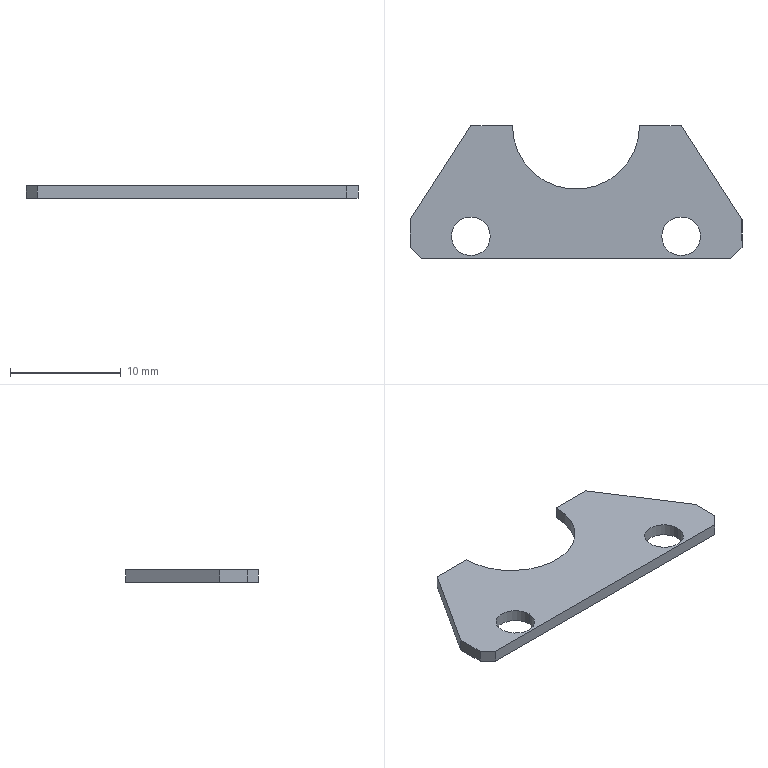Part | STEP file | 11-FG-SB00511 | 1 solid | 16 faces | box 30 x 12 x 1.1 mm | volume 265.181 mm3 | plane 11 | cylinder 5 | commonest cylinder face diameters 3.5 x4 11.5 x1
STEP:
#1=CARTESIAN_POINT('',(11.25,-4.,1.1));
#2=VERTEX_POINT('',#1);
#3=CARTESIAN_POINT('',(7.75,-4.,1.1));
#4=VERTEX_POINT('',#3);
#5=CARTESIAN_POINT('',(9.5,-4.,1.1));
#6=DIRECTION('',(0.,0.,-1.));
#7=DIRECTION('',(1.,0.,0.));
#8=AXIS2_PLACEMENT_3D('',#5,#6,#7);
#9=CIRCLE('',#8,1.75);
#10=EDGE_CURVE('',#2,#4,#9,.T.);
#11=ORIENTED_EDGE('',*,*,#10,.F.);
#12=CARTESIAN_POINT('',(11.25,-4.,0.));
#13=VERTEX_POINT('',#12);
#14=CARTESIAN_POINT('',(11.25,-4.,1.1));
#15=DIRECTION('',(0.,0.,-1.));
#16=VECTOR('',#15,1000.);
#17=LINE('',#14,#16);
#18=EDGE_CURVE('',#2,#13,#17,.T.);
#19=ORIENTED_EDGE('',*,*,#18,.T.);
#20=CARTESIAN_POINT('',(7.75,-4.,0.));
#21=VERTEX_POINT('',#20);
#22=CARTESIAN_POINT('',(9.5,-4.,0.));
#23=DIRECTION('',(0.,0.,1.));
#24=DIRECTION('',(1.,0.,0.));
#25=AXIS2_PLACEMENT_3D('',#22,#23,#24);
#26=CIRCLE('',#25,1.75);
#27=EDGE_CURVE('',#21,#13,#26,.T.);
#28=ORIENTED_EDGE('',*,*,#27,.F.);
#29=CARTESIAN_POINT('',(7.75,-4.,1.1));
#30=DIRECTION('',(0.,0.,-1.));
#31=VECTOR('',#30,1000.);
#32=LINE('',#29,#31);
#33=EDGE_CURVE('',#4,#21,#32,.T.);
#34=ORIENTED_EDGE('',*,*,#33,.F.);
#35=EDGE_LOOP('',(#11,#19,#28,#34));
#36=FACE_OUTER_BOUND('',#35,.T.);
#37=CARTESIAN_POINT('',(9.5,-4.,1.1));
#38=DIRECTION('',(0.,0.,-1.));
#39=DIRECTION('',(-1.,0.,0.));
#40=AXIS2_PLACEMENT_3D('',#37,#38,#39);
#41=CYLINDRICAL_SURFACE('',#40,1.75);
#42=ADVANCED_FACE('',(#36),#41,.F.);
#43=CARTESIAN_POINT('',(-7.75,-4.,1.1));
#44=VERTEX_POINT('',#43);
#45=CARTESIAN_POINT('',(-11.25,-4.,1.1));
#46=VERTEX_POINT('',#45);
#47=CARTESIAN_POINT('',(-9.5,-4.,1.1));
#48=DIRECTION('',(0.,0.,-1.));
#49=DIRECTION('',(-1.,0.,0.));
#50=AXIS2_PLACEMENT_3D('',#47,#48,#49);
#51=CIRCLE('',#50,1.75);
#52=EDGE_CURVE('',#44,#46,#51,.T.);
#53=ORIENTED_EDGE('',*,*,#52,.F.);
#54=CARTESIAN_POINT('',(-7.75,-4.,0.));
#55=VERTEX_POINT('',#54);
#56=CARTESIAN_POINT('',(-7.75,-4.,1.1));
#57=DIRECTION('',(0.,0.,-1.));
#58=VECTOR('',#57,1000.);
#59=LINE('',#56,#58);
#60=EDGE_CURVE('',#44,#55,#59,.T.);
#61=ORIENTED_EDGE('',*,*,#60,.T.);
#62=CARTESIAN_POINT('',(-11.25,-4.,0.));
#63=VERTEX_POINT('',#62);
#64=CARTESIAN_POINT('',(-9.5,-4.,0.));
#65=DIRECTION('',(0.,0.,1.));
#66=DIRECTION('',(1.,0.,0.));
#67=AXIS2_PLACEMENT_3D('',#64,#65,#66);
#68=CIRCLE('',#67,1.75);
#69=EDGE_CURVE('',#63,#55,#68,.T.);
#70=ORIENTED_EDGE('',*,*,#69,.F.);
#71=CARTESIAN_POINT('',(-11.25,-4.,1.1));
#72=DIRECTION('',(0.,0.,-1.));
#73=VECTOR('',#72,1000.);
#74=LINE('',#71,#73);
#75=EDGE_CURVE('',#46,#63,#74,.T.);
#76=ORIENTED_EDGE('',*,*,#75,.F.);
#77=EDGE_LOOP('',(#53,#61,#70,#76));
#78=FACE_OUTER_BOUND('',#77,.T.);
#79=CARTESIAN_POINT('',(-9.5,-4.,1.1));
#80=DIRECTION('',(0.,0.,-1.));
#81=DIRECTION('',(-1.,0.,0.));
#82=AXIS2_PLACEMENT_3D('',#79,#80,#81);
#83=CYLINDRICAL_SURFACE('',#82,1.75);
#84=ADVANCED_FACE('',(#78),#83,.F.);
#85=CARTESIAN_POINT('',(9.5,6.,1.1));
#86=VERTEX_POINT('',#85);
#87=CARTESIAN_POINT('',(5.75,6.,1.1));
#88=VERTEX_POINT('',#87);
#89=CARTESIAN_POINT('',(-15.,6.,1.1));
#90=DIRECTION('',(-1.,0.,0.));
#91=VECTOR('',#90,1000.);
#92=LINE('',#89,#91);
#93=EDGE_CURVE('',#86,#88,#92,.T.);
#94=ORIENTED_EDGE('',*,*,#93,.F.);
#95=CARTESIAN_POINT('',(9.5,6.,0.));
#96=VERTEX_POINT('',#95);
#97=CARTESIAN_POINT('',(9.5,6.,1.1));
#98=DIRECTION('',(0.,0.,-1.));
#99=VECTOR('',#98,1000.);
#100=LINE('',#97,#99);
#101=EDGE_CURVE('',#86,#96,#100,.T.);
#102=ORIENTED_EDGE('',*,*,#101,.T.);
#103=CARTESIAN_POINT('',(5.75,6.,0.));
#104=VERTEX_POINT('',#103);
#105=CARTESIAN_POINT('',(-15.,6.,0.));
#106=DIRECTION('',(-1.,0.,0.));
#107=VECTOR('',#106,1000.);
#108=LINE('',#105,#107);
#109=EDGE_CURVE('',#96,#104,#108,.T.);
#110=ORIENTED_EDGE('',*,*,#109,.T.);
#111=CARTESIAN_POINT('',(5.75,6.,0.));
#112=DIRECTION('',(0.,0.,1.));
#113=VECTOR('',#112,1000.);
#114=LINE('',#111,#113);
#115=EDGE_CURVE('',#104,#88,#114,.T.);
#116=ORIENTED_EDGE('',*,*,#115,.T.);
#117=EDGE_LOOP('',(#94,#102,#110,#116));
#118=FACE_OUTER_BOUND('',#117,.T.);
#119=CARTESIAN_POINT('',(-15.,6.,1.1));
#120=DIRECTION('',(0.,-1.,0.));
#121=DIRECTION('',(0.,0.,-1.));
#122=AXIS2_PLACEMENT_3D('',#119,#120,#121);
#123=PLANE('',#122);
#124=ADVANCED_FACE('',(#118),#123,.F.);
#125=CARTESIAN_POINT('',(15.,-5.,0.));
#126=VERTEX_POINT('',#125);
#127=CARTESIAN_POINT('',(15.,-2.5,0.));
#128=VERTEX_POINT('',#127);
#129=CARTESIAN_POINT('',(15.,6.,0.));
#130=DIRECTION('',(0.,1.,0.));
#131=VECTOR('',#130,1000.);
#132=LINE('',#129,#131);
#133=EDGE_CURVE('',#126,#128,#132,.T.);
#134=ORIENTED_EDGE('',*,*,#133,.T.);
#135=CARTESIAN_POINT('',(15.,-2.5,1.1));
#136=VERTEX_POINT('',#135);
#137=CARTESIAN_POINT('',(15.,-2.5,1.1));
#138=DIRECTION('',(0.,0.,-1.));
#139=VECTOR('',#138,1000.);
#140=LINE('',#137,#139);
#141=EDGE_CURVE('',#136,#128,#140,.T.);
#142=ORIENTED_EDGE('',*,*,#141,.F.);
#143=CARTESIAN_POINT('',(15.,-5.,1.1));
#144=VERTEX_POINT('',#143);
#145=CARTESIAN_POINT('',(15.,6.,1.1));
#146=DIRECTION('',(0.,1.,0.));
#147=VECTOR('',#146,1000.);
#148=LINE('',#145,#147);
#149=EDGE_CURVE('',#144,#136,#148,.T.);
#150=ORIENTED_EDGE('',*,*,#149,.F.);
#151=CARTESIAN_POINT('',(15.,-5.,1.1));
#152=DIRECTION('',(0.,0.,-1.));
#153=VECTOR('',#152,1000.);
#154=LINE('',#151,#153);
#155=EDGE_CURVE('',#144,#126,#154,.T.);
#156=ORIENTED_EDGE('',*,*,#155,.T.);
#157=EDGE_LOOP('',(#134,#142,#150,#156));
#158=FACE_OUTER_BOUND('',#157,.T.);
#159=CARTESIAN_POINT('',(15.,6.,1.1));
#160=DIRECTION('',(-1.,0.,0.));
#161=DIRECTION('',(0.,-1.,0.));
#162=AXIS2_PLACEMENT_3D('',#159,#160,#161);
#163=PLANE('',#162);
#164=ADVANCED_FACE('',(#158),#163,.F.);
#165=CARTESIAN_POINT('',(-5.75,6.,0.));
#166=VERTEX_POINT('',#165);
#167=CARTESIAN_POINT('',(-9.5,6.,0.));
#168=VERTEX_POINT('',#167);
#169=CARTESIAN_POINT('',(-15.,6.,0.));
#170=DIRECTION('',(-1.,0.,0.));
#171=VECTOR('',#170,1000.);
#172=LINE('',#169,#171);
#173=EDGE_CURVE('',#166,#168,#172,.T.);
#174=ORIENTED_EDGE('',*,*,#173,.T.);
#175=CARTESIAN_POINT('',(-9.5,6.,1.1));
#176=VERTEX_POINT('',#175);
#177=CARTESIAN_POINT('',(-9.5,6.,1.1));
#178=DIRECTION('',(0.,0.,-1.));
#179=VECTOR('',#178,1000.);
#180=LINE('',#177,#179);
#181=EDGE_CURVE('',#176,#168,#180,.T.);
#182=ORIENTED_EDGE('',*,*,#181,.F.);
#183=CARTESIAN_POINT('',(-5.75,6.,1.1));
#184=VERTEX_POINT('',#183);
#185=CARTESIAN_POINT('',(-15.,6.,1.1));
#186=DIRECTION('',(-1.,0.,0.));
#187=VECTOR('',#186,1000.);
#188=LINE('',#185,#187);
#189=EDGE_CURVE('',#184,#176,#188,.T.);
#190=ORIENTED_EDGE('',*,*,#189,.F.);
#191=CARTESIAN_POINT('',(-5.75,6.,0.));
#192=DIRECTION('',(0.,0.,-1.));
#193=VECTOR('',#192,1000.);
#194=LINE('',#191,#193);
#195=EDGE_CURVE('',#184,#166,#194,.T.);
#196=ORIENTED_EDGE('',*,*,#195,.T.);
#197=EDGE_LOOP('',(#174,#182,#190,#196));
#198=FACE_OUTER_BOUND('',#197,.T.);
#199=CARTESIAN_POINT('',(-15.,6.,1.1));
#200=DIRECTION('',(0.,-1.,0.));
#201=DIRECTION('',(0.,0.,-1.));
#202=AXIS2_PLACEMENT_3D('',#199,#200,#201);
#203=PLANE('',#202);
#204=ADVANCED_FACE('',(#198),#203,.F.);
#205=CARTESIAN_POINT('',(-15.,-2.5,1.1));
#206=VERTEX_POINT('',#205);
#207=CARTESIAN_POINT('',(-15.,-5.,1.1));
#208=VERTEX_POINT('',#207);
#209=CARTESIAN_POINT('',(-15.,6.,1.1));
#210=DIRECTION('',(0.,-1.,0.));
#211=VECTOR('',#210,1000.);
#212=LINE('',#209,#211);
#213=EDGE_CURVE('',#206,#208,#212,.T.);
#214=ORIENTED_EDGE('',*,*,#213,.F.);
#215=CARTESIAN_POINT('',(-15.,-2.5,0.));
#216=VERTEX_POINT('',#215);
#217=CARTESIAN_POINT('',(-15.,-2.5,1.1));
#218=DIRECTION('',(0.,0.,-1.));
#219=VECTOR('',#218,1000.);
#220=LINE('',#217,#219);
#221=EDGE_CURVE('',#206,#216,#220,.T.);
#222=ORIENTED_EDGE('',*,*,#221,.T.);
#223=CARTESIAN_POINT('',(-15.,-5.,0.));
#224=VERTEX_POINT('',#223);
#225=CARTESIAN_POINT('',(-15.,6.,0.));
#226=DIRECTION('',(0.,-1.,0.));
#227=VECTOR('',#226,1000.);
#228=LINE('',#225,#227);
#229=EDGE_CURVE('',#216,#224,#228,.T.);
#230=ORIENTED_EDGE('',*,*,#229,.T.);
#231=CARTESIAN_POINT('',(-15.,-5.,1.1));
#232=DIRECTION('',(0.,0.,1.));
#233=VECTOR('',#232,1000.);
#234=LINE('',#231,#233);
#235=EDGE_CURVE('',#224,#208,#234,.T.);
#236=ORIENTED_EDGE('',*,*,#235,.T.);
#237=EDGE_LOOP('',(#214,#222,#230,#236));
#238=FACE_OUTER_BOUND('',#237,.T.);
#239=CARTESIAN_POINT('',(-15.,6.,1.1));
#240=DIRECTION('',(1.,0.,0.));
#241=DIRECTION('',(0.,1.,0.));
#242=AXIS2_PLACEMENT_3D('',#239,#240,#241);
#243=PLANE('',#242);
#244=ADVANCED_FACE('',(#238),#243,.F.);
#245=CARTESIAN_POINT('',(-14.,-6.,1.1));
#246=VERTEX_POINT('',#245);
#247=CARTESIAN_POINT('',(14.,-6.,1.1));
#248=VERTEX_POINT('',#247);
#249=CARTESIAN_POINT('',(-15.,-6.,1.1));
#250=DIRECTION('',(1.,0.,0.));
#251=VECTOR('',#250,1000.);
#252=LINE('',#249,#251);
#253=EDGE_CURVE('',#246,#248,#252,.T.);
#254=ORIENTED_EDGE('',*,*,#253,.F.);
#255=CARTESIAN_POINT('',(-14.,-6.,0.));
#256=VERTEX_POINT('',#255);
#257=CARTESIAN_POINT('',(-14.,-6.,1.1));
#258=DIRECTION('',(0.,0.,-1.));
#259=VECTOR('',#258,1000.);
#260=LINE('',#257,#259);
#261=EDGE_CURVE('',#246,#256,#260,.T.);
#262=ORIENTED_EDGE('',*,*,#261,.T.);
#263=CARTESIAN_POINT('',(14.,-6.,0.));
#264=VERTEX_POINT('',#263);
#265=CARTESIAN_POINT('',(-15.,-6.,0.));
#266=DIRECTION('',(1.,0.,0.));
#267=VECTOR('',#266,1000.);
#268=LINE('',#265,#267);
#269=EDGE_CURVE('',#256,#264,#268,.T.);
#270=ORIENTED_EDGE('',*,*,#269,.T.);
#271=CARTESIAN_POINT('',(14.,-6.,1.1));
#272=DIRECTION('',(0.,0.,1.));
#273=VECTOR('',#272,1000.);
#274=LINE('',#271,#273);
#275=EDGE_CURVE('',#264,#248,#274,.T.);
#276=ORIENTED_EDGE('',*,*,#275,.T.);
#277=EDGE_LOOP('',(#254,#262,#270,#276));
#278=FACE_OUTER_BOUND('',#277,.T.);
#279=CARTESIAN_POINT('',(-15.,-6.,1.1));
#280=DIRECTION('',(0.,1.,0.));
#281=DIRECTION('',(0.,0.,1.));
#282=AXIS2_PLACEMENT_3D('',#279,#280,#281);
#283=PLANE('',#282);
#284=ADVANCED_FACE('',(#278),#283,.F.);
#285=CARTESIAN_POINT('',(9.5,-4.,1.1));
#286=DIRECTION('',(0.,0.,-1.));
#287=DIRECTION('',(1.,0.,0.));
#288=AXIS2_PLACEMENT_3D('',#285,#286,#287);
#289=CIRCLE('',#288,1.75);
#290=EDGE_CURVE('',#4,#2,#289,.T.);
#291=ORIENTED_EDGE('',*,*,#290,.T.);
#292=ORIENTED_EDGE('',*,*,#10,.T.);
#293=EDGE_LOOP('',(#291,#292));
#294=FACE_BOUND('',#293,.T.);
#295=CARTESIAN_POINT('',(-9.5,-4.,1.1));
#296=DIRECTION('',(0.,0.,-1.));
#297=DIRECTION('',(-1.,0.,0.));
#298=AXIS2_PLACEMENT_3D('',#295,#296,#297);
#299=CIRCLE('',#298,1.75);
#300=EDGE_CURVE('',#46,#44,#299,.T.);
#301=ORIENTED_EDGE('',*,*,#300,.T.);
#302=ORIENTED_EDGE('',*,*,#52,.T.);
#303=EDGE_LOOP('',(#301,#302));
#304=FACE_BOUND('',#303,.T.);
#305=CARTESIAN_POINT('',(15.,-2.5,1.1));
#306=DIRECTION('',(-0.5433,0.8396,0.));
#307=VECTOR('',#306,1000.);
#308=LINE('',#305,#307);
#309=EDGE_CURVE('',#136,#86,#308,.T.);
#310=ORIENTED_EDGE('',*,*,#309,.T.);
#311=ORIENTED_EDGE('',*,*,#93,.T.);
#312=CARTESIAN_POINT('',(0.,6.,1.1));
#313=DIRECTION('',(0.,0.,1.));
#314=DIRECTION('',(1.,0.,0.));
#315=AXIS2_PLACEMENT_3D('',#312,#313,#314);
#316=CIRCLE('',#315,5.75);
#317=EDGE_CURVE('',#184,#88,#316,.T.);
#318=ORIENTED_EDGE('',*,*,#317,.F.);
#319=ORIENTED_EDGE('',*,*,#189,.T.);
#320=CARTESIAN_POINT('',(-15.,-2.5,1.1));
#321=DIRECTION('',(-0.5433,-0.8396,0.));
#322=VECTOR('',#321,1000.);
#323=LINE('',#320,#322);
#324=EDGE_CURVE('',#176,#206,#323,.T.);
#325=ORIENTED_EDGE('',*,*,#324,.T.);
#326=ORIENTED_EDGE('',*,*,#213,.T.);
#327=CARTESIAN_POINT('',(-10.,-10.,1.1));
#328=DIRECTION('',(0.7071,-0.7071,0.));
#329=VECTOR('',#328,1000.);
#330=LINE('',#327,#329);
#331=EDGE_CURVE('',#208,#246,#330,.T.);
#332=ORIENTED_EDGE('',*,*,#331,.T.);
#333=ORIENTED_EDGE('',*,*,#253,.T.);
#334=CARTESIAN_POINT('',(10.,-10.,1.1));
#335=DIRECTION('',(0.7071,0.7071,0.));
#336=VECTOR('',#335,1000.);
#337=LINE('',#334,#336);
#338=EDGE_CURVE('',#248,#144,#337,.T.);
#339=ORIENTED_EDGE('',*,*,#338,.T.);
#340=ORIENTED_EDGE('',*,*,#149,.T.);
#341=EDGE_LOOP('',(#310,#311,#318,#319,#325,#326,#332,#333,#339,#340));
#342=FACE_OUTER_BOUND('',#341,.T.);
#343=CARTESIAN_POINT('',(0.,0.,1.1));
#344=DIRECTION('',(0.,0.,1.));
#345=DIRECTION('',(1.,0.,0.));
#346=AXIS2_PLACEMENT_3D('',#343,#344,#345);
#347=PLANE('',#346);
#348=ADVANCED_FACE('',(#294,#304,#342),#347,.T.);
#349=ORIENTED_EDGE('',*,*,#27,.T.);
#350=CARTESIAN_POINT('',(9.5,-4.,0.));
#351=DIRECTION('',(0.,0.,1.));
#352=DIRECTION('',(1.,0.,0.));
#353=AXIS2_PLACEMENT_3D('',#350,#351,#352);
#354=CIRCLE('',#353,1.75);
#355=EDGE_CURVE('',#13,#21,#354,.T.);
#356=ORIENTED_EDGE('',*,*,#355,.T.);
#357=EDGE_LOOP('',(#349,#356));
#358=FACE_BOUND('',#357,.T.);
#359=ORIENTED_EDGE('',*,*,#69,.T.);
#360=CARTESIAN_POINT('',(-9.5,-4.,0.));
#361=DIRECTION('',(0.,0.,1.));
#362=DIRECTION('',(1.,0.,0.));
#363=AXIS2_PLACEMENT_3D('',#360,#361,#362);
#364=CIRCLE('',#363,1.75);
#365=EDGE_CURVE('',#55,#63,#364,.T.);
#366=ORIENTED_EDGE('',*,*,#365,.T.);
#367=EDGE_LOOP('',(#359,#366));
#368=FACE_BOUND('',#367,.T.);
#369=ORIENTED_EDGE('',*,*,#109,.F.);
#370=CARTESIAN_POINT('',(15.,-2.5,0.));
#371=DIRECTION('',(-0.5433,0.8396,0.));
#372=VECTOR('',#371,1000.);
#373=LINE('',#370,#372);
#374=EDGE_CURVE('',#128,#96,#373,.T.);
#375=ORIENTED_EDGE('',*,*,#374,.F.);
#376=ORIENTED_EDGE('',*,*,#133,.F.);
#377=CARTESIAN_POINT('',(15.,-5.,0.));
#378=DIRECTION('',(-0.7071,-0.7071,0.));
#379=VECTOR('',#378,1000.);
#380=LINE('',#377,#379);
#381=EDGE_CURVE('',#126,#264,#380,.T.);
#382=ORIENTED_EDGE('',*,*,#381,.T.);
#383=ORIENTED_EDGE('',*,*,#269,.F.);
#384=CARTESIAN_POINT('',(-14.,-6.,0.));
#385=DIRECTION('',(-0.7071,0.7071,0.));
#386=VECTOR('',#385,1000.);
#387=LINE('',#384,#386);
#388=EDGE_CURVE('',#256,#224,#387,.T.);
#389=ORIENTED_EDGE('',*,*,#388,.T.);
#390=ORIENTED_EDGE('',*,*,#229,.F.);
#391=CARTESIAN_POINT('',(-15.,-2.5,0.));
#392=DIRECTION('',(-0.5433,-0.8396,0.));
#393=VECTOR('',#392,1000.);
#394=LINE('',#391,#393);
#395=EDGE_CURVE('',#168,#216,#394,.T.);
#396=ORIENTED_EDGE('',*,*,#395,.F.);
#397=ORIENTED_EDGE('',*,*,#173,.F.);
#398=CARTESIAN_POINT('',(0.,6.,0.));
#399=DIRECTION('',(0.,0.,1.));
#400=DIRECTION('',(1.,0.,0.));
#401=AXIS2_PLACEMENT_3D('',#398,#399,#400);
#402=CIRCLE('',#401,5.75);
#403=EDGE_CURVE('',#166,#104,#402,.T.);
#404=ORIENTED_EDGE('',*,*,#403,.T.);
#405=EDGE_LOOP('',(#369,#375,#376,#382,#383,#389,#390,#396,#397,#404));
#406=FACE_OUTER_BOUND('',#405,.T.);
#407=CARTESIAN_POINT('',(0.,0.,0.));
#408=DIRECTION('',(0.,0.,1.));
#409=DIRECTION('',(1.,0.,0.));
#410=AXIS2_PLACEMENT_3D('',#407,#408,#409);
#411=PLANE('',#410);
#412=ADVANCED_FACE('',(#358,#368,#406),#411,.F.);
#413=ORIENTED_EDGE('',*,*,#403,.F.);
#414=ORIENTED_EDGE('',*,*,#195,.F.);
#415=ORIENTED_EDGE('',*,*,#317,.T.);
#416=ORIENTED_EDGE('',*,*,#115,.F.);
#417=EDGE_LOOP('',(#413,#414,#415,#416));
#418=FACE_OUTER_BOUND('',#417,.T.);
#419=CARTESIAN_POINT('',(0.,6.,0.));
#420=DIRECTION('',(0.,0.,1.));
#421=DIRECTION('',(1.,0.,0.));
#422=AXIS2_PLACEMENT_3D('',#419,#420,#421);
#423=CYLINDRICAL_SURFACE('',#422,5.75);
#424=ADVANCED_FACE('',(#418),#423,.F.);
#425=ORIENTED_EDGE('',*,*,#331,.F.);
#426=ORIENTED_EDGE('',*,*,#235,.F.);
#427=ORIENTED_EDGE('',*,*,#388,.F.);
#428=ORIENTED_EDGE('',*,*,#261,.F.);
#429=EDGE_LOOP('',(#425,#426,#427,#428));
#430=FACE_OUTER_BOUND('',#429,.T.);
#431=CARTESIAN_POINT('',(-14.,-6.,1.1));
#432=DIRECTION('',(0.7071,0.7071,0.));
#433=DIRECTION('',(0.,0.,-1.));
#434=AXIS2_PLACEMENT_3D('',#431,#432,#433);
#435=PLANE('',#434);
#436=ADVANCED_FACE('',(#430),#435,.F.);
#437=ORIENTED_EDGE('',*,*,#338,.F.);
#438=ORIENTED_EDGE('',*,*,#275,.F.);
#439=ORIENTED_EDGE('',*,*,#381,.F.);
#440=ORIENTED_EDGE('',*,*,#155,.F.);
#441=EDGE_LOOP('',(#437,#438,#439,#440));
#442=FACE_OUTER_BOUND('',#441,.T.);
#443=CARTESIAN_POINT('',(15.,-5.,1.1));
#444=DIRECTION('',(-0.7071,0.7071,0.));
#445=DIRECTION('',(0.,0.,-1.));
#446=AXIS2_PLACEMENT_3D('',#443,#444,#445);
#447=PLANE('',#446);
#448=ADVANCED_FACE('',(#442),#447,.F.);
#449=ORIENTED_EDGE('',*,*,#395,.T.);
#450=ORIENTED_EDGE('',*,*,#221,.F.);
#451=ORIENTED_EDGE('',*,*,#324,.F.);
#452=ORIENTED_EDGE('',*,*,#181,.T.);
#453=EDGE_LOOP('',(#449,#450,#451,#452));
#454=FACE_OUTER_BOUND('',#453,.T.);
#455=CARTESIAN_POINT('',(-15.,-2.5,1.1));
#456=DIRECTION('',(0.8396,-0.5433,0.));
#457=DIRECTION('',(0.5433,0.8396,0.));
#458=AXIS2_PLACEMENT_3D('',#455,#456,#457);
#459=PLANE('',#458);
#460=ADVANCED_FACE('',(#454),#459,.F.);
#461=ORIENTED_EDGE('',*,*,#374,.T.);
#462=ORIENTED_EDGE('',*,*,#101,.F.);
#463=ORIENTED_EDGE('',*,*,#309,.F.);
#464=ORIENTED_EDGE('',*,*,#141,.T.);
#465=EDGE_LOOP('',(#461,#462,#463,#464));
#466=FACE_OUTER_BOUND('',#465,.T.);
#467=CARTESIAN_POINT('',(15.,-2.5,1.1));
#468=DIRECTION('',(-0.8396,-0.5433,0.));
#469=DIRECTION('',(0.5433,-0.8396,0.));
#470=AXIS2_PLACEMENT_3D('',#467,#468,#469);
#471=PLANE('',#470);
#472=ADVANCED_FACE('',(#466),#471,.F.);
#473=ORIENTED_EDGE('',*,*,#60,.F.);
#474=ORIENTED_EDGE('',*,*,#300,.F.);
#475=ORIENTED_EDGE('',*,*,#75,.T.);
#476=ORIENTED_EDGE('',*,*,#365,.F.);
#477=EDGE_LOOP('',(#473,#474,#475,#476));
#478=FACE_OUTER_BOUND('',#477,.T.);
#479=CARTESIAN_POINT('',(-9.5,-4.,1.1));
#480=DIRECTION('',(0.,0.,-1.));
#481=DIRECTION('',(-1.,0.,0.));
#482=AXIS2_PLACEMENT_3D('',#479,#480,#481);
#483=CYLINDRICAL_SURFACE('',#482,1.75);
#484=ADVANCED_FACE('',(#478),#483,.F.);
#485=ORIENTED_EDGE('',*,*,#18,.F.);
#486=ORIENTED_EDGE('',*,*,#290,.F.);
#487=ORIENTED_EDGE('',*,*,#33,.T.);
#488=ORIENTED_EDGE('',*,*,#355,.F.);
#489=EDGE_LOOP('',(#485,#486,#487,#488));
#490=FACE_OUTER_BOUND('',#489,.T.);
#491=CARTESIAN_POINT('',(9.5,-4.,1.1));
#492=DIRECTION('',(0.,0.,-1.));
#493=DIRECTION('',(-1.,0.,0.));
#494=AXIS2_PLACEMENT_3D('',#491,#492,#493);
#495=CYLINDRICAL_SURFACE('',#494,1.75);
#496=ADVANCED_FACE('',(#490),#495,.F.);
#497=CLOSED_SHELL('',(#42,#84,#124,#164,#204,#244,#284,#348,#412,#424,#436,#448,#460,#472,#484,#496));
#498=MANIFOLD_SOLID_BREP('',#497);
#499=CARTESIAN_POINT('',(0.,0.,0.));
#500=DIRECTION('',(0.,0.,1.));
#501=DIRECTION('',(1.,0.,0.));
#502=AXIS2_PLACEMENT_3D('',#499,#500,#501);
#503=(LENGTH_UNIT()NAMED_UNIT(*)SI_UNIT(.MILLI.,.METRE.));
#504=UNCERTAINTY_MEASURE_WITH_UNIT(LENGTH_MEASURE(0.00001),#503,'','');
#505=(NAMED_UNIT(*)PLANE_ANGLE_UNIT()SI_UNIT($,.RADIAN.));
#506=(NAMED_UNIT(*)SI_UNIT($,.STERADIAN.)SOLID_ANGLE_UNIT());
#507=(GEOMETRIC_REPRESENTATION_CONTEXT(3)GLOBAL_UNCERTAINTY_ASSIGNED_CONTEXT((#504))GLOBAL_UNIT_ASSIGNED_CONTEXT((#503,#505,#506))REPRESENTATION_CONTEXT('',''));
#508=ADVANCED_BREP_SHAPE_REPRESENTATION('',(#498,#502),#507);